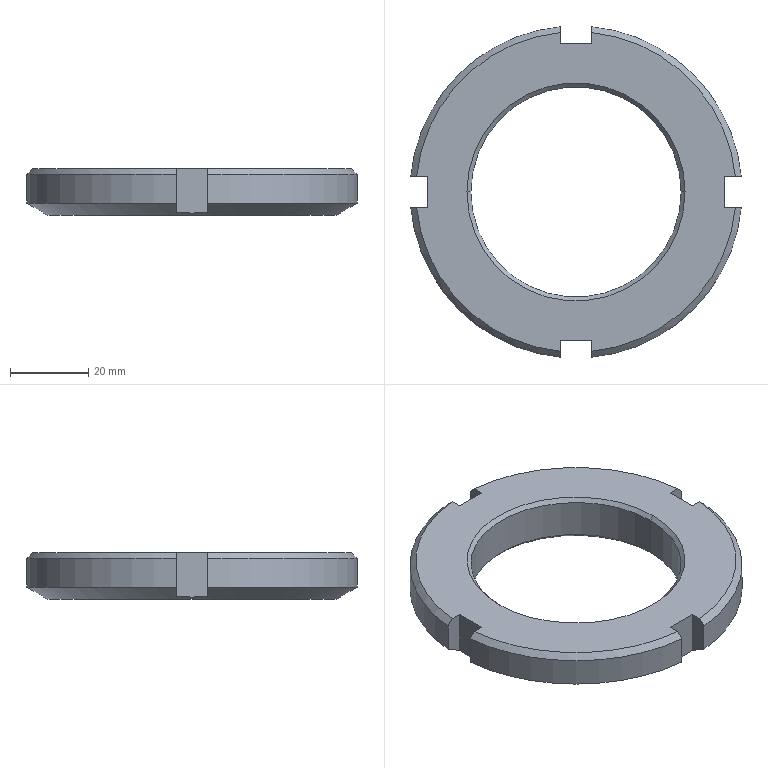Part | SolidWorks | features Chamfer 3, CirPattern 1, Cut 1, Extrusion 1 | 1 solid | 30 faces | box 84.623 x 84.623 x 12 mm | volume 36703 mm3 | plane 14 | cone 10 | cylinder 6 | commonest cylinder face diameters 85 x4 53.835 x2
STEP:
#1=CARTESIAN_POINT('',(-26.918,0.,11.));
#2=VERTEX_POINT('',#1);
#3=CARTESIAN_POINT('',(26.918,0.,11.));
#4=VERTEX_POINT('',#3);
#5=CARTESIAN_POINT('',(0.,0.,11.));
#6=DIRECTION('',(0.,0.,1.));
#7=DIRECTION('',(1.,0.,0.));
#8=AXIS2_PLACEMENT_3D('',#5,#6,#7);
#9=CIRCLE('',#8,26.918);
#10=EDGE_CURVE('',#2,#4,#9,.T.);
#11=ORIENTED_EDGE('',*,*,#10,.F.);
#12=CARTESIAN_POINT('',(-27.917,0.,12.));
#13=VERTEX_POINT('',#12);
#14=CARTESIAN_POINT('',(-26.918,0.,11.));
#15=DIRECTION('',(-0.7071,0.,0.7071));
#16=VECTOR('',#15,1000.);
#17=LINE('',#14,#16);
#18=EDGE_CURVE('',#2,#13,#17,.T.);
#19=ORIENTED_EDGE('',*,*,#18,.T.);
#20=CARTESIAN_POINT('',(27.917,0.,12.));
#21=VERTEX_POINT('',#20);
#22=CARTESIAN_POINT('',(0.,0.,12.));
#23=DIRECTION('',(0.,0.,-1.));
#24=DIRECTION('',(1.,0.,0.));
#25=AXIS2_PLACEMENT_3D('',#22,#23,#24);
#26=CIRCLE('',#25,27.917);
#27=EDGE_CURVE('',#21,#13,#26,.T.);
#28=ORIENTED_EDGE('',*,*,#27,.F.);
#29=CARTESIAN_POINT('',(26.918,0.,11.));
#30=DIRECTION('',(0.7071,0.,0.7071));
#31=VECTOR('',#30,1000.);
#32=LINE('',#29,#31);
#33=EDGE_CURVE('',#4,#21,#32,.T.);
#34=ORIENTED_EDGE('',*,*,#33,.F.);
#35=EDGE_LOOP('',(#11,#19,#28,#34));
#36=FACE_OUTER_BOUND('',#35,.T.);
#37=CARTESIAN_POINT('',(0.,0.,11.));
#38=DIRECTION('',(0.,0.,1.));
#39=DIRECTION('',(1.,0.,0.));
#40=AXIS2_PLACEMENT_3D('',#37,#38,#39);
#41=CONICAL_SURFACE('',#40,26.918,0.7854);
#42=ADVANCED_FACE('',(#36),#41,.F.);
#43=CARTESIAN_POINT('',(26.918,0.,1.));
#44=VERTEX_POINT('',#43);
#45=CARTESIAN_POINT('',(-26.918,0.,1.));
#46=VERTEX_POINT('',#45);
#47=CARTESIAN_POINT('',(0.,0.,1.));
#48=DIRECTION('',(0.,0.,-1.));
#49=DIRECTION('',(1.,0.,0.));
#50=AXIS2_PLACEMENT_3D('',#47,#48,#49);
#51=CIRCLE('',#50,26.918);
#52=EDGE_CURVE('',#44,#46,#51,.T.);
#53=ORIENTED_EDGE('',*,*,#52,.F.);
#54=CARTESIAN_POINT('',(27.917,0.,0.));
#55=VERTEX_POINT('',#54);
#56=CARTESIAN_POINT('',(27.917,0.,0.));
#57=DIRECTION('',(0.7071,0.,-0.7071));
#58=VECTOR('',#57,1000.);
#59=LINE('',#56,#58);
#60=EDGE_CURVE('',#44,#55,#59,.T.);
#61=ORIENTED_EDGE('',*,*,#60,.T.);
#62=CARTESIAN_POINT('',(-27.917,0.,0.));
#63=VERTEX_POINT('',#62);
#64=CARTESIAN_POINT('',(0.,0.,0.));
#65=DIRECTION('',(0.,0.,1.));
#66=DIRECTION('',(1.,0.,0.));
#67=AXIS2_PLACEMENT_3D('',#64,#65,#66);
#68=CIRCLE('',#67,27.917);
#69=EDGE_CURVE('',#63,#55,#68,.T.);
#70=ORIENTED_EDGE('',*,*,#69,.F.);
#71=CARTESIAN_POINT('',(-27.917,0.,0.));
#72=DIRECTION('',(-0.7071,0.,-0.7071));
#73=VECTOR('',#72,1000.);
#74=LINE('',#71,#73);
#75=EDGE_CURVE('',#46,#63,#74,.T.);
#76=ORIENTED_EDGE('',*,*,#75,.F.);
#77=EDGE_LOOP('',(#53,#61,#70,#76));
#78=FACE_OUTER_BOUND('',#77,.T.);
#79=CARTESIAN_POINT('',(0.,0.,0.));
#80=DIRECTION('',(0.,0.,-1.));
#81=DIRECTION('',(-1.,0.,0.));
#82=AXIS2_PLACEMENT_3D('',#79,#80,#81);
#83=CONICAL_SURFACE('',#82,27.917,0.7854);
#84=ADVANCED_FACE('',(#78),#83,.F.);
#85=CARTESIAN_POINT('',(-37.,0.,0.));
#86=VERTEX_POINT('',#85);
#87=CARTESIAN_POINT('',(37.,0.,0.));
#88=VERTEX_POINT('',#87);
#89=CARTESIAN_POINT('',(0.,0.,0.));
#90=DIRECTION('',(0.,0.,-1.));
#91=DIRECTION('',(1.,0.,0.));
#92=AXIS2_PLACEMENT_3D('',#89,#90,#91);
#93=CIRCLE('',#92,37.);
#94=EDGE_CURVE('',#86,#88,#93,.T.);
#95=ORIENTED_EDGE('',*,*,#94,.F.);
#96=CARTESIAN_POINT('',(-38.061,0.,0.6128));
#97=VERTEX_POINT('',#96);
#98=CARTESIAN_POINT('',(-42.5,0.,3.175));
#99=DIRECTION('',(-0.866,0.,0.5));
#100=VECTOR('',#99,1000.);
#101=LINE('',#98,#100);
#102=EDGE_CURVE('',#86,#97,#101,.T.);
#103=ORIENTED_EDGE('',*,*,#102,.T.);
#104=CARTESIAN_POINT('',(-38.061,4.,0.7338));
#105=VERTEX_POINT('',#104);
#106=CARTESIAN_POINT('',(-38.061,4.,0.7338));
#107=CARTESIAN_POINT('',(-38.061,2.67,0.6535));
#108=CARTESIAN_POINT('',(-38.061,1.337,0.6128));
#109=CARTESIAN_POINT('',(-38.061,0.,0.6128));
#110=B_SPLINE_CURVE_WITH_KNOTS('',3,(#106,#107,#108,#109),.UNSPECIFIED.,.F.,.F.,(4,4),(0.01039,0.01438),.UNSPECIFIED.);
#111=EDGE_CURVE('',#105,#97,#110,.T.);
#112=ORIENTED_EDGE('',*,*,#111,.F.);
#113=CARTESIAN_POINT('',(-42.311,4.,3.175));
#114=VERTEX_POINT('',#113);
#115=CARTESIAN_POINT('',(-42.311,4.,3.175));
#116=CARTESIAN_POINT('',(-42.064,4.,3.033));
#117=CARTESIAN_POINT('',(-41.816,4.,2.891));
#118=CARTESIAN_POINT('',(-41.569,4.,2.749));
#119=CARTESIAN_POINT('',(-40.4,4.,2.077));
#120=CARTESIAN_POINT('',(-39.231,4.,1.405));
#121=CARTESIAN_POINT('',(-38.061,4.,0.7338));
#122=B_SPLINE_CURVE_WITH_KNOTS('',3,(#115,#116,#117,#118,#119,#120,#121),.UNSPECIFIED.,.F.,.F.,(4,3,4),(0.009231,0.01009,0.01413),.UNSPECIFIED.);
#123=EDGE_CURVE('',#114,#105,#122,.T.);
#124=ORIENTED_EDGE('',*,*,#123,.F.);
#125=CARTESIAN_POINT('',(-4.,42.311,3.175));
#126=VERTEX_POINT('',#125);
#127=CARTESIAN_POINT('',(0.,0.,3.175));
#128=DIRECTION('',(0.,0.,1.));
#129=DIRECTION('',(1.,0.,0.));
#130=AXIS2_PLACEMENT_3D('',#127,#128,#129);
#131=CIRCLE('',#130,42.5);
#132=EDGE_CURVE('',#126,#114,#131,.T.);
#133=ORIENTED_EDGE('',*,*,#132,.F.);
#134=CARTESIAN_POINT('',(-4.,38.061,0.7338));
#135=VERTEX_POINT('',#134);
#136=CARTESIAN_POINT('',(-4.,38.061,0.7338));
#137=CARTESIAN_POINT('',(-4.,38.203,0.8152));
#138=CARTESIAN_POINT('',(-4.,38.345,0.8967));
#139=CARTESIAN_POINT('',(-4.,38.487,0.9781));
#140=CARTESIAN_POINT('',(-4.,39.762,1.71));
#141=CARTESIAN_POINT('',(-4.,41.037,2.443));
#142=CARTESIAN_POINT('',(-4.,42.311,3.175));
#143=B_SPLINE_CURVE_WITH_KNOTS('',3,(#136,#137,#138,#139,#140,#141,#142),.UNSPECIFIED.,.F.,.F.,(4,3,4),(0.009597,0.01009,0.0145),.UNSPECIFIED.);
#144=EDGE_CURVE('',#135,#126,#143,.T.);
#145=ORIENTED_EDGE('',*,*,#144,.F.);
#146=CARTESIAN_POINT('',(4.,38.061,0.7338));
#147=VERTEX_POINT('',#146);
#148=CARTESIAN_POINT('',(4.,38.061,0.7338));
#149=CARTESIAN_POINT('',(2.673,38.061,0.6537));
#150=CARTESIAN_POINT('',(1.343,38.061,0.613));
#151=CARTESIAN_POINT('',(-1.324,38.061,0.6126));
#152=CARTESIAN_POINT('',(-2.664,38.061,0.6532));
#153=CARTESIAN_POINT('',(-4.,38.061,0.7338));
#154=B_SPLINE_CURVE_WITH_KNOTS('',3,(#148,#149,#150,#151,#152,#153),.UNSPECIFIED.,.F.,.F.,(4,2,4),(0.01039,0.01437,0.01836),.UNSPECIFIED.);
#155=EDGE_CURVE('',#147,#135,#154,.T.);
#156=ORIENTED_EDGE('',*,*,#155,.F.);
#157=CARTESIAN_POINT('',(4.,42.311,3.175));
#158=VERTEX_POINT('',#157);
#159=CARTESIAN_POINT('',(4.,42.311,3.175));
#160=CARTESIAN_POINT('',(4.,41.037,2.443));
#161=CARTESIAN_POINT('',(4.,39.762,1.71));
#162=CARTESIAN_POINT('',(4.,38.487,0.9781));
#163=CARTESIAN_POINT('',(4.,38.345,0.8967));
#164=CARTESIAN_POINT('',(4.,38.203,0.8152));
#165=CARTESIAN_POINT('',(4.,38.061,0.7338));
#166=B_SPLINE_CURVE_WITH_KNOTS('',3,(#159,#160,#161,#162,#163,#164,#165),.UNSPECIFIED.,.F.,.F.,(4,3,4),(0.005677,0.01009,0.01058),.UNSPECIFIED.);
#167=EDGE_CURVE('',#158,#147,#166,.T.);
#168=ORIENTED_EDGE('',*,*,#167,.F.);
#169=CARTESIAN_POINT('',(42.311,4.,3.175));
#170=VERTEX_POINT('',#169);
#171=CARTESIAN_POINT('',(0.,0.,3.175));
#172=DIRECTION('',(0.,0.,1.));
#173=DIRECTION('',(1.,0.,0.));
#174=AXIS2_PLACEMENT_3D('',#171,#172,#173);
#175=CIRCLE('',#174,42.5);
#176=EDGE_CURVE('',#170,#158,#175,.T.);
#177=ORIENTED_EDGE('',*,*,#176,.F.);
#178=CARTESIAN_POINT('',(38.061,4.,0.7338));
#179=VERTEX_POINT('',#178);
#180=CARTESIAN_POINT('',(38.061,4.,0.7338));
#181=CARTESIAN_POINT('',(38.203,4.,0.8152));
#182=CARTESIAN_POINT('',(38.345,4.,0.8967));
#183=CARTESIAN_POINT('',(38.487,4.,0.9781));
#184=CARTESIAN_POINT('',(39.762,4.,1.71));
#185=CARTESIAN_POINT('',(41.037,4.,2.443));
#186=CARTESIAN_POINT('',(42.311,4.,3.175));
#187=B_SPLINE_CURVE_WITH_KNOTS('',3,(#180,#181,#182,#183,#184,#185,#186),.UNSPECIFIED.,.F.,.F.,(4,3,4),(0.009597,0.01009,0.0145),.UNSPECIFIED.);
#188=EDGE_CURVE('',#179,#170,#187,.T.);
#189=ORIENTED_EDGE('',*,*,#188,.F.);
#190=CARTESIAN_POINT('',(38.061,0.,0.6128));
#191=VERTEX_POINT('',#190);
#192=CARTESIAN_POINT('',(38.061,0.,0.6128));
#193=CARTESIAN_POINT('',(38.061,1.337,0.6128));
#194=CARTESIAN_POINT('',(38.061,2.67,0.6535));
#195=CARTESIAN_POINT('',(38.061,4.,0.7338));
#196=B_SPLINE_CURVE_WITH_KNOTS('',3,(#192,#193,#194,#195),.UNSPECIFIED.,.F.,.F.,(4,4),(0.02042,0.02442),.UNSPECIFIED.);
#197=EDGE_CURVE('',#191,#179,#196,.T.);
#198=ORIENTED_EDGE('',*,*,#197,.F.);
#199=CARTESIAN_POINT('',(42.5,0.,3.175));
#200=DIRECTION('',(0.866,0.,0.5));
#201=VECTOR('',#200,1000.);
#202=LINE('',#199,#201);
#203=EDGE_CURVE('',#88,#191,#202,.T.);
#204=ORIENTED_EDGE('',*,*,#203,.F.);
#205=EDGE_LOOP('',(#95,#103,#112,#124,#133,#145,#156,#168,#177,#189,#198,#204));
#206=FACE_OUTER_BOUND('',#205,.T.);
#207=CARTESIAN_POINT('',(0.,0.,3.175));
#208=DIRECTION('',(0.,0.,1.));
#209=DIRECTION('',(1.,0.,0.));
#210=AXIS2_PLACEMENT_3D('',#207,#208,#209);
#211=CONICAL_SURFACE('',#210,42.5,1.047);
#212=ADVANCED_FACE('',(#206),#211,.T.);
#213=ORIENTED_EDGE('',*,*,#10,.T.);
#214=CARTESIAN_POINT('',(26.918,0.,12.));
#215=DIRECTION('',(0.,0.,-1.));
#216=VECTOR('',#215,1000.);
#217=LINE('',#214,#216);
#218=EDGE_CURVE('',#4,#44,#217,.T.);
#219=ORIENTED_EDGE('',*,*,#218,.T.);
#220=ORIENTED_EDGE('',*,*,#52,.T.);
#221=CARTESIAN_POINT('',(-26.918,0.,12.));
#222=DIRECTION('',(0.,0.,-1.));
#223=VECTOR('',#222,1000.);
#224=LINE('',#221,#223);
#225=EDGE_CURVE('',#2,#46,#224,.T.);
#226=ORIENTED_EDGE('',*,*,#225,.F.);
#227=EDGE_LOOP('',(#213,#219,#220,#226));
#228=FACE_OUTER_BOUND('',#227,.T.);
#229=CARTESIAN_POINT('',(0.,0.,12.));
#230=DIRECTION('',(0.,0.,-1.));
#231=DIRECTION('',(-1.,0.,0.));
#232=AXIS2_PLACEMENT_3D('',#229,#230,#231);
#233=CYLINDRICAL_SURFACE('',#232,26.918);
#234=ADVANCED_FACE('',(#228),#233,.F.);
#235=CARTESIAN_POINT('',(4.,42.311,10.5));
#236=VERTEX_POINT('',#235);
#237=CARTESIAN_POINT('',(42.311,4.,10.5));
#238=VERTEX_POINT('',#237);
#239=CARTESIAN_POINT('',(0.,0.,10.5));
#240=DIRECTION('',(0.,0.,-1.));
#241=DIRECTION('',(1.,0.,0.));
#242=AXIS2_PLACEMENT_3D('',#239,#240,#241);
#243=CIRCLE('',#242,42.5);
#244=EDGE_CURVE('',#236,#238,#243,.T.);
#245=ORIENTED_EDGE('',*,*,#244,.T.);
#246=CARTESIAN_POINT('',(42.311,4.,0.));
#247=DIRECTION('',(0.,0.,1.));
#248=VECTOR('',#247,1000.);
#249=LINE('',#246,#248);
#250=EDGE_CURVE('',#170,#238,#249,.T.);
#251=ORIENTED_EDGE('',*,*,#250,.F.);
#252=ORIENTED_EDGE('',*,*,#176,.T.);
#253=CARTESIAN_POINT('',(4.,42.311,0.));
#254=DIRECTION('',(0.,0.,1.));
#255=VECTOR('',#254,1000.);
#256=LINE('',#253,#255);
#257=EDGE_CURVE('',#158,#236,#256,.T.);
#258=ORIENTED_EDGE('',*,*,#257,.T.);
#259=EDGE_LOOP('',(#245,#251,#252,#258));
#260=FACE_OUTER_BOUND('',#259,.T.);
#261=CARTESIAN_POINT('',(0.,0.,12.));
#262=DIRECTION('',(0.,0.,-1.));
#263=DIRECTION('',(-1.,0.,0.));
#264=AXIS2_PLACEMENT_3D('',#261,#262,#263);
#265=CYLINDRICAL_SURFACE('',#264,42.5);
#266=ADVANCED_FACE('',(#260),#265,.T.);
#267=CARTESIAN_POINT('',(40.804,4.,12.));
#268=VERTEX_POINT('',#267);
#269=CARTESIAN_POINT('',(42.311,4.,10.5));
#270=CARTESIAN_POINT('',(41.92,4.,10.89));
#271=CARTESIAN_POINT('',(41.528,4.,11.28));
#272=CARTESIAN_POINT('',(41.136,4.,11.67));
#273=CARTESIAN_POINT('',(41.025,4.,11.78));
#274=CARTESIAN_POINT('',(40.915,4.,11.89));
#275=CARTESIAN_POINT('',(40.804,4.,12.));
#276=B_SPLINE_CURVE_WITH_KNOTS('',3,(#269,#270,#271,#272,#273,#274,#275),.UNSPECIFIED.,.F.,.F.,(4,3,4),(0.007217,0.008875,0.009343),.UNSPECIFIED.);
#277=EDGE_CURVE('',#238,#268,#276,.T.);
#278=ORIENTED_EDGE('',*,*,#277,.F.);
#279=ORIENTED_EDGE('',*,*,#244,.F.);
#280=CARTESIAN_POINT('',(4.,40.804,12.));
#281=VERTEX_POINT('',#280);
#282=CARTESIAN_POINT('',(4.,40.804,12.));
#283=CARTESIAN_POINT('',(4.,40.915,11.89));
#284=CARTESIAN_POINT('',(4.,41.025,11.78));
#285=CARTESIAN_POINT('',(4.,41.136,11.67));
#286=CARTESIAN_POINT('',(4.,41.528,11.28));
#287=CARTESIAN_POINT('',(4.,41.92,10.89));
#288=CARTESIAN_POINT('',(4.,42.311,10.5));
#289=B_SPLINE_CURVE_WITH_KNOTS('',3,(#282,#283,#284,#285,#286,#287,#288),.UNSPECIFIED.,.F.,.F.,(4,3,4),(0.008408,0.008875,0.01053),.UNSPECIFIED.);
#290=EDGE_CURVE('',#281,#236,#289,.T.);
#291=ORIENTED_EDGE('',*,*,#290,.F.);
#292=CARTESIAN_POINT('',(0.,0.,12.));
#293=DIRECTION('',(0.,0.,1.));
#294=DIRECTION('',(1.,0.,0.));
#295=AXIS2_PLACEMENT_3D('',#292,#293,#294);
#296=CIRCLE('',#295,41.);
#297=EDGE_CURVE('',#268,#281,#296,.T.);
#298=ORIENTED_EDGE('',*,*,#297,.F.);
#299=EDGE_LOOP('',(#278,#279,#291,#298));
#300=FACE_OUTER_BOUND('',#299,.T.);
#301=CARTESIAN_POINT('',(0.,0.,12.));
#302=DIRECTION('',(0.,0.,-1.));
#303=DIRECTION('',(-1.,0.,0.));
#304=AXIS2_PLACEMENT_3D('',#301,#302,#303);
#305=CONICAL_SURFACE('',#304,41.,0.7854);
#306=ADVANCED_FACE('',(#300),#305,.T.);
#307=CARTESIAN_POINT('',(-42.311,4.,10.5));
#308=VERTEX_POINT('',#307);
#309=CARTESIAN_POINT('',(-4.,42.311,10.5));
#310=VERTEX_POINT('',#309);
#311=CARTESIAN_POINT('',(0.,0.,10.5));
#312=DIRECTION('',(0.,0.,-1.));
#313=DIRECTION('',(1.,0.,0.));
#314=AXIS2_PLACEMENT_3D('',#311,#312,#313);
#315=CIRCLE('',#314,42.5);
#316=EDGE_CURVE('',#308,#310,#315,.T.);
#317=ORIENTED_EDGE('',*,*,#316,.T.);
#318=CARTESIAN_POINT('',(-4.,42.311,0.));
#319=DIRECTION('',(0.,0.,1.));
#320=VECTOR('',#319,1000.);
#321=LINE('',#318,#320);
#322=EDGE_CURVE('',#126,#310,#321,.T.);
#323=ORIENTED_EDGE('',*,*,#322,.F.);
#324=ORIENTED_EDGE('',*,*,#132,.T.);
#325=CARTESIAN_POINT('',(-42.311,4.,0.));
#326=DIRECTION('',(0.,0.,1.));
#327=VECTOR('',#326,1000.);
#328=LINE('',#325,#327);
#329=EDGE_CURVE('',#114,#308,#328,.T.);
#330=ORIENTED_EDGE('',*,*,#329,.T.);
#331=EDGE_LOOP('',(#317,#323,#324,#330));
#332=FACE_OUTER_BOUND('',#331,.T.);
#333=CARTESIAN_POINT('',(0.,0.,12.));
#334=DIRECTION('',(0.,0.,-1.));
#335=DIRECTION('',(-1.,0.,0.));
#336=AXIS2_PLACEMENT_3D('',#333,#334,#335);
#337=CYLINDRICAL_SURFACE('',#336,42.5);
#338=ADVANCED_FACE('',(#332),#337,.T.);
#339=CARTESIAN_POINT('',(-4.,40.804,12.));
#340=VERTEX_POINT('',#339);
#341=CARTESIAN_POINT('',(-4.,42.311,10.5));
#342=CARTESIAN_POINT('',(-4.,41.92,10.89));
#343=CARTESIAN_POINT('',(-4.,41.528,11.28));
#344=CARTESIAN_POINT('',(-4.,41.136,11.67));
#345=CARTESIAN_POINT('',(-4.,41.025,11.78));
#346=CARTESIAN_POINT('',(-4.,40.915,11.89));
#347=CARTESIAN_POINT('',(-4.,40.804,12.));
#348=B_SPLINE_CURVE_WITH_KNOTS('',3,(#341,#342,#343,#344,#345,#346,#347),.UNSPECIFIED.,.F.,.F.,(4,3,4),(0.007217,0.008875,0.009343),.UNSPECIFIED.);
#349=EDGE_CURVE('',#310,#340,#348,.T.);
#350=ORIENTED_EDGE('',*,*,#349,.F.);
#351=ORIENTED_EDGE('',*,*,#316,.F.);
#352=CARTESIAN_POINT('',(-40.804,4.,12.));
#353=VERTEX_POINT('',#352);
#354=CARTESIAN_POINT('',(-40.804,4.,12.));
#355=CARTESIAN_POINT('',(-41.093,4.,11.713));
#356=CARTESIAN_POINT('',(-41.381,4.,11.426));
#357=CARTESIAN_POINT('',(-41.67,4.,11.139));
#358=CARTESIAN_POINT('',(-41.883,4.,10.926));
#359=CARTESIAN_POINT('',(-42.097,4.,10.713));
#360=CARTESIAN_POINT('',(-42.311,4.,10.5));
#361=B_SPLINE_CURVE_WITH_KNOTS('',3,(#354,#355,#356,#357,#358,#359,#360),.UNSPECIFIED.,.F.,.F.,(4,3,4),(0.007655,0.008875,0.009781),.UNSPECIFIED.);
#362=EDGE_CURVE('',#353,#308,#361,.T.);
#363=ORIENTED_EDGE('',*,*,#362,.F.);
#364=CARTESIAN_POINT('',(0.,0.,12.));
#365=DIRECTION('',(0.,0.,1.));
#366=DIRECTION('',(1.,0.,0.));
#367=AXIS2_PLACEMENT_3D('',#364,#365,#366);
#368=CIRCLE('',#367,41.);
#369=EDGE_CURVE('',#340,#353,#368,.T.);
#370=ORIENTED_EDGE('',*,*,#369,.F.);
#371=EDGE_LOOP('',(#350,#351,#363,#370));
#372=FACE_OUTER_BOUND('',#371,.T.);
#373=CARTESIAN_POINT('',(0.,0.,12.));
#374=DIRECTION('',(0.,0.,-1.));
#375=DIRECTION('',(-1.,0.,0.));
#376=AXIS2_PLACEMENT_3D('',#373,#374,#375);
#377=CONICAL_SURFACE('',#376,41.,0.7854);
#378=ADVANCED_FACE('',(#372),#377,.T.);
#379=CARTESIAN_POINT('',(-4.,-42.311,10.5));
#380=VERTEX_POINT('',#379);
#381=CARTESIAN_POINT('',(-42.311,-4.,10.5));
#382=VERTEX_POINT('',#381);
#383=CARTESIAN_POINT('',(0.,0.,10.5));
#384=DIRECTION('',(0.,0.,-1.));
#385=DIRECTION('',(1.,0.,0.));
#386=AXIS2_PLACEMENT_3D('',#383,#384,#385);
#387=CIRCLE('',#386,42.5);
#388=EDGE_CURVE('',#380,#382,#387,.T.);
#389=ORIENTED_EDGE('',*,*,#388,.T.);
#390=CARTESIAN_POINT('',(-42.311,-4.,3.175));
#391=VERTEX_POINT('',#390);
#392=CARTESIAN_POINT('',(-42.311,-4.,0.));
#393=DIRECTION('',(0.,0.,1.));
#394=VECTOR('',#393,1000.);
#395=LINE('',#392,#394);
#396=EDGE_CURVE('',#391,#382,#395,.T.);
#397=ORIENTED_EDGE('',*,*,#396,.F.);
#398=CARTESIAN_POINT('',(-4.,-42.311,3.175));
#399=VERTEX_POINT('',#398);
#400=CARTESIAN_POINT('',(0.,0.,3.175));
#401=DIRECTION('',(0.,0.,1.));
#402=DIRECTION('',(1.,0.,0.));
#403=AXIS2_PLACEMENT_3D('',#400,#401,#402);
#404=CIRCLE('',#403,42.5);
#405=EDGE_CURVE('',#391,#399,#404,.T.);
#406=ORIENTED_EDGE('',*,*,#405,.T.);
#407=CARTESIAN_POINT('',(-4.,-42.311,0.));
#408=DIRECTION('',(0.,0.,1.));
#409=VECTOR('',#408,1000.);
#410=LINE('',#407,#409);
#411=EDGE_CURVE('',#399,#380,#410,.T.);
#412=ORIENTED_EDGE('',*,*,#411,.T.);
#413=EDGE_LOOP('',(#389,#397,#406,#412));
#414=FACE_OUTER_BOUND('',#413,.T.);
#415=CARTESIAN_POINT('',(0.,0.,12.));
#416=DIRECTION('',(0.,0.,-1.));
#417=DIRECTION('',(-1.,0.,0.));
#418=AXIS2_PLACEMENT_3D('',#415,#416,#417);
#419=CYLINDRICAL_SURFACE('',#418,42.5);
#420=ADVANCED_FACE('',(#414),#419,.T.);
#421=CARTESIAN_POINT('',(-40.804,-4.,12.));
#422=VERTEX_POINT('',#421);
#423=CARTESIAN_POINT('',(-42.311,-4.,10.5));
#424=CARTESIAN_POINT('',(-42.097,-4.,10.713));
#425=CARTESIAN_POINT('',(-41.883,-4.,10.926));
#426=CARTESIAN_POINT('',(-41.67,-4.,11.139));
#427=CARTESIAN_POINT('',(-41.381,-4.,11.426));
#428=CARTESIAN_POINT('',(-41.093,-4.,11.713));
#429=CARTESIAN_POINT('',(-40.804,-4.,12.));
#430=B_SPLINE_CURVE_WITH_KNOTS('',3,(#423,#424,#425,#426,#427,#428,#429),.UNSPECIFIED.,.F.,.F.,(4,3,4),(0.00797,0.008875,0.0101),.UNSPECIFIED.);
#431=EDGE_CURVE('',#382,#422,#430,.T.);
#432=ORIENTED_EDGE('',*,*,#431,.F.);
#433=ORIENTED_EDGE('',*,*,#388,.F.);
#434=CARTESIAN_POINT('',(-4.,-40.804,12.));
#435=VERTEX_POINT('',#434);
#436=CARTESIAN_POINT('',(-4.,-40.804,12.));
#437=CARTESIAN_POINT('',(-4.,-41.093,11.713));
#438=CARTESIAN_POINT('',(-4.,-41.381,11.426));
#439=CARTESIAN_POINT('',(-4.,-41.67,11.139));
#440=CARTESIAN_POINT('',(-4.,-41.883,10.926));
#441=CARTESIAN_POINT('',(-4.,-42.097,10.713));
#442=CARTESIAN_POINT('',(-4.,-42.311,10.5));
#443=B_SPLINE_CURVE_WITH_KNOTS('',3,(#436,#437,#438,#439,#440,#441,#442),.UNSPECIFIED.,.F.,.F.,(4,3,4),(0.007655,0.008875,0.009781),.UNSPECIFIED.);
#444=EDGE_CURVE('',#435,#380,#443,.T.);
#445=ORIENTED_EDGE('',*,*,#444,.F.);
#446=CARTESIAN_POINT('',(0.,0.,12.));
#447=DIRECTION('',(0.,0.,1.));
#448=DIRECTION('',(1.,0.,0.));
#449=AXIS2_PLACEMENT_3D('',#446,#447,#448);
#450=CIRCLE('',#449,41.);
#451=EDGE_CURVE('',#422,#435,#450,.T.);
#452=ORIENTED_EDGE('',*,*,#451,.F.);
#453=EDGE_LOOP('',(#432,#433,#445,#452));
#454=FACE_OUTER_BOUND('',#453,.T.);
#455=CARTESIAN_POINT('',(0.,0.,12.));
#456=DIRECTION('',(0.,0.,-1.));
#457=DIRECTION('',(-1.,0.,0.));
#458=AXIS2_PLACEMENT_3D('',#455,#456,#457);
#459=CONICAL_SURFACE('',#458,41.,0.7854);
#460=ADVANCED_FACE('',(#454),#459,.T.);
#461=ORIENTED_EDGE('',*,*,#27,.T.);
#462=CARTESIAN_POINT('',(0.,0.,12.));
#463=DIRECTION('',(0.,0.,-1.));
#464=DIRECTION('',(1.,0.,0.));
#465=AXIS2_PLACEMENT_3D('',#462,#463,#464);
#466=CIRCLE('',#465,27.917);
#467=EDGE_CURVE('',#13,#21,#466,.T.);
#468=ORIENTED_EDGE('',*,*,#467,.T.);
#469=EDGE_LOOP('',(#461,#468));
#470=FACE_BOUND('',#469,.T.);
#471=CARTESIAN_POINT('',(38.061,4.,12.));
#472=VERTEX_POINT('',#471);
#473=CARTESIAN_POINT('',(38.061,4.,12.));
#474=DIRECTION('',(-1.,0.,0.));
#475=VECTOR('',#474,1000.);
#476=LINE('',#473,#475);
#477=EDGE_CURVE('',#268,#472,#476,.T.);
#478=ORIENTED_EDGE('',*,*,#477,.F.);
#479=ORIENTED_EDGE('',*,*,#297,.T.);
#480=CARTESIAN_POINT('',(4.,38.061,12.));
#481=VERTEX_POINT('',#480);
#482=CARTESIAN_POINT('',(4.,38.061,12.));
#483=DIRECTION('',(0.,1.,0.));
#484=VECTOR('',#483,1000.);
#485=LINE('',#482,#484);
#486=EDGE_CURVE('',#481,#281,#485,.T.);
#487=ORIENTED_EDGE('',*,*,#486,.F.);
#488=CARTESIAN_POINT('',(-4.,38.061,12.));
#489=VERTEX_POINT('',#488);
#490=CARTESIAN_POINT('',(4.,38.061,12.));
#491=DIRECTION('',(1.,0.,0.));
#492=VECTOR('',#491,1000.);
#493=LINE('',#490,#492);
#494=EDGE_CURVE('',#489,#481,#493,.T.);
#495=ORIENTED_EDGE('',*,*,#494,.F.);
#496=CARTESIAN_POINT('',(-4.,38.061,12.));
#497=DIRECTION('',(0.,-1.,0.));
#498=VECTOR('',#497,1000.);
#499=LINE('',#496,#498);
#500=EDGE_CURVE('',#340,#489,#499,.T.);
#501=ORIENTED_EDGE('',*,*,#500,.F.);
#502=ORIENTED_EDGE('',*,*,#369,.T.);
#503=CARTESIAN_POINT('',(-38.061,4.,12.));
#504=VERTEX_POINT('',#503);
#505=CARTESIAN_POINT('',(-38.061,4.,12.));
#506=DIRECTION('',(-1.,0.,0.));
#507=VECTOR('',#506,1000.);
#508=LINE('',#505,#507);
#509=EDGE_CURVE('',#504,#353,#508,.T.);
#510=ORIENTED_EDGE('',*,*,#509,.F.);
#511=CARTESIAN_POINT('',(-38.061,-4.,12.));
#512=VERTEX_POINT('',#511);
#513=CARTESIAN_POINT('',(-38.061,4.,12.));
#514=DIRECTION('',(0.,1.,0.));
#515=VECTOR('',#514,1000.);
#516=LINE('',#513,#515);
#517=EDGE_CURVE('',#512,#504,#516,.T.);
#518=ORIENTED_EDGE('',*,*,#517,.F.);
#519=CARTESIAN_POINT('',(-38.061,-4.,12.));
#520=DIRECTION('',(1.,0.,0.));
#521=VECTOR('',#520,1000.);
#522=LINE('',#519,#521);
#523=EDGE_CURVE('',#422,#512,#522,.T.);
#524=ORIENTED_EDGE('',*,*,#523,.F.);
#525=ORIENTED_EDGE('',*,*,#451,.T.);
#526=CARTESIAN_POINT('',(-4.,-38.061,12.));
#527=VERTEX_POINT('',#526);
#528=CARTESIAN_POINT('',(-4.,-38.061,12.));
#529=DIRECTION('',(0.,-1.,0.));
#530=VECTOR('',#529,1000.);
#531=LINE('',#528,#530);
#532=EDGE_CURVE('',#527,#435,#531,.T.);
#533=ORIENTED_EDGE('',*,*,#532,.F.);
#534=CARTESIAN_POINT('',(4.,-38.061,12.));
#535=VERTEX_POINT('',#534);
#536=CARTESIAN_POINT('',(-4.,-38.061,12.));
#537=DIRECTION('',(-1.,0.,0.));
#538=VECTOR('',#537,1000.);
#539=LINE('',#536,#538);
#540=EDGE_CURVE('',#535,#527,#539,.T.);
#541=ORIENTED_EDGE('',*,*,#540,.F.);
#542=CARTESIAN_POINT('',(4.,-40.804,12.));
#543=VERTEX_POINT('',#542);
#544=CARTESIAN_POINT('',(4.,-38.061,12.));
#545=DIRECTION('',(0.,1.,0.));
#546=VECTOR('',#545,1000.);
#547=LINE('',#544,#546);
#548=EDGE_CURVE('',#543,#535,#547,.T.);
#549=ORIENTED_EDGE('',*,*,#548,.F.);
#550=CARTESIAN_POINT('',(40.804,-4.,12.));
#551=VERTEX_POINT('',#550);
#552=CARTESIAN_POINT('',(0.,0.,12.));
#553=DIRECTION('',(0.,0.,1.));
#554=DIRECTION('',(1.,0.,0.));
#555=AXIS2_PLACEMENT_3D('',#552,#553,#554);
#556=CIRCLE('',#555,41.);
#557=EDGE_CURVE('',#543,#551,#556,.T.);
#558=ORIENTED_EDGE('',*,*,#557,.T.);
#559=CARTESIAN_POINT('',(38.061,-4.,12.));
#560=VERTEX_POINT('',#559);
#561=CARTESIAN_POINT('',(38.061,-4.,12.));
#562=DIRECTION('',(1.,0.,0.));
#563=VECTOR('',#562,1000.);
#564=LINE('',#561,#563);
#565=EDGE_CURVE('',#560,#551,#564,.T.);
#566=ORIENTED_EDGE('',*,*,#565,.F.);
#567=CARTESIAN_POINT('',(38.061,-4.,12.));
#568=DIRECTION('',(0.,-1.,0.));
#569=VECTOR('',#568,1000.);
#570=LINE('',#567,#569);
#571=EDGE_CURVE('',#472,#560,#570,.T.);
#572=ORIENTED_EDGE('',*,*,#571,.F.);
#573=EDGE_LOOP('',(#478,#479,#487,#495,#501,#502,#510,#518,#524,#525,#533,#541,#549,#558,#566,#572));
#574=FACE_OUTER_BOUND('',#573,.T.);
#575=CARTESIAN_POINT('',(0.,0.,12.));
#576=DIRECTION('',(0.,0.,1.));
#577=DIRECTION('',(1.,0.,0.));
#578=AXIS2_PLACEMENT_3D('',#575,#576,#577);
#579=PLANE('',#578);
#580=ADVANCED_FACE('',(#470,#574),#579,.T.);
#581=ORIENTED_EDGE('',*,*,#69,.T.);
#582=CARTESIAN_POINT('',(0.,0.,0.));
#583=DIRECTION('',(0.,0.,1.));
#584=DIRECTION('',(1.,0.,0.));
#585=AXIS2_PLACEMENT_3D('',#582,#583,#584);
#586=CIRCLE('',#585,27.917);
#587=EDGE_CURVE('',#55,#63,#586,.T.);
#588=ORIENTED_EDGE('',*,*,#587,.T.);
#589=EDGE_LOOP('',(#581,#588));
#590=FACE_BOUND('',#589,.T.);
#591=CARTESIAN_POINT('',(0.,0.,0.));
#592=DIRECTION('',(0.,0.,-1.));
#593=DIRECTION('',(1.,0.,0.));
#594=AXIS2_PLACEMENT_3D('',#591,#592,#593);
#595=CIRCLE('',#594,37.);
#596=EDGE_CURVE('',#88,#86,#595,.T.);
#597=ORIENTED_EDGE('',*,*,#596,.T.);
#598=ORIENTED_EDGE('',*,*,#94,.T.);
#599=EDGE_LOOP('',(#597,#598));
#600=FACE_OUTER_BOUND('',#599,.T.);
#601=CARTESIAN_POINT('',(0.,0.,0.));
#602=DIRECTION('',(0.,0.,1.));
#603=DIRECTION('',(1.,0.,0.));
#604=AXIS2_PLACEMENT_3D('',#601,#602,#603);
#605=PLANE('',#604);
#606=ADVANCED_FACE('',(#590,#600),#605,.F.);
#607=CARTESIAN_POINT('',(4.,-42.311,3.175));
#608=VERTEX_POINT('',#607);
#609=CARTESIAN_POINT('',(42.311,-4.,3.175));
#610=VERTEX_POINT('',#609);
#611=CARTESIAN_POINT('',(0.,0.,3.175));
#612=DIRECTION('',(0.,0.,1.));
#613=DIRECTION('',(1.,0.,0.));
#614=AXIS2_PLACEMENT_3D('',#611,#612,#613);
#615=CIRCLE('',#614,42.5);
#616=EDGE_CURVE('',#608,#610,#615,.T.);
#617=ORIENTED_EDGE('',*,*,#616,.T.);
#618=CARTESIAN_POINT('',(42.311,-4.,10.5));
#619=VERTEX_POINT('',#618);
#620=CARTESIAN_POINT('',(42.311,-4.,0.));
#621=DIRECTION('',(0.,0.,1.));
#622=VECTOR('',#621,1000.);
#623=LINE('',#620,#622);
#624=EDGE_CURVE('',#610,#619,#623,.T.);
#625=ORIENTED_EDGE('',*,*,#624,.T.);
#626=CARTESIAN_POINT('',(4.,-42.311,10.5));
#627=VERTEX_POINT('',#626);
#628=CARTESIAN_POINT('',(0.,0.,10.5));
#629=DIRECTION('',(0.,0.,-1.));
#630=DIRECTION('',(1.,0.,0.));
#631=AXIS2_PLACEMENT_3D('',#628,#629,#630);
#632=CIRCLE('',#631,42.5);
#633=EDGE_CURVE('',#619,#627,#632,.T.);
#634=ORIENTED_EDGE('',*,*,#633,.T.);
#635=CARTESIAN_POINT('',(4.,-42.311,0.));
#636=DIRECTION('',(0.,0.,1.));
#637=VECTOR('',#636,1000.);
#638=LINE('',#635,#637);
#639=EDGE_CURVE('',#608,#627,#638,.T.);
#640=ORIENTED_EDGE('',*,*,#639,.F.);
#641=EDGE_LOOP('',(#617,#625,#634,#640));
#642=FACE_OUTER_BOUND('',#641,.T.);
#643=CARTESIAN_POINT('',(0.,0.,12.));
#644=DIRECTION('',(0.,0.,-1.));
#645=DIRECTION('',(-1.,0.,0.));
#646=AXIS2_PLACEMENT_3D('',#643,#644,#645);
#647=CYLINDRICAL_SURFACE('',#646,42.5);
#648=ADVANCED_FACE('',(#642),#647,.T.);
#649=ORIENTED_EDGE('',*,*,#218,.F.);
#650=CARTESIAN_POINT('',(0.,0.,11.));
#651=DIRECTION('',(0.,0.,1.));
#652=DIRECTION('',(1.,0.,0.));
#653=AXIS2_PLACEMENT_3D('',#650,#651,#652);
#654=CIRCLE('',#653,26.918);
#655=EDGE_CURVE('',#4,#2,#654,.T.);
#656=ORIENTED_EDGE('',*,*,#655,.T.);
#657=ORIENTED_EDGE('',*,*,#225,.T.);
#658=CARTESIAN_POINT('',(0.,0.,1.));
#659=DIRECTION('',(0.,0.,-1.));
#660=DIRECTION('',(1.,0.,0.));
#661=AXIS2_PLACEMENT_3D('',#658,#659,#660);
#662=CIRCLE('',#661,26.918);
#663=EDGE_CURVE('',#46,#44,#662,.T.);
#664=ORIENTED_EDGE('',*,*,#663,.T.);
#665=EDGE_LOOP('',(#649,#656,#657,#664));
#666=FACE_OUTER_BOUND('',#665,.T.);
#667=CARTESIAN_POINT('',(0.,0.,12.));
#668=DIRECTION('',(0.,0.,-1.));
#669=DIRECTION('',(-1.,0.,0.));
#670=AXIS2_PLACEMENT_3D('',#667,#668,#669);
#671=CYLINDRICAL_SURFACE('',#670,26.918);
#672=ADVANCED_FACE('',(#666),#671,.F.);
#673=CARTESIAN_POINT('',(40.804,-4.,12.));
#674=CARTESIAN_POINT('',(40.915,-4.,11.89));
#675=CARTESIAN_POINT('',(41.025,-4.,11.78));
#676=CARTESIAN_POINT('',(41.136,-4.,11.67));
#677=CARTESIAN_POINT('',(41.528,-4.,11.28));
#678=CARTESIAN_POINT('',(41.92,-4.,10.89));
#679=CARTESIAN_POINT('',(42.311,-4.,10.5));
#680=B_SPLINE_CURVE_WITH_KNOTS('',3,(#673,#674,#675,#676,#677,#678,#679),.UNSPECIFIED.,.F.,.F.,(4,3,4),(0.008408,0.008875,0.01053),.UNSPECIFIED.);
#681=EDGE_CURVE('',#551,#619,#680,.T.);
#682=ORIENTED_EDGE('',*,*,#681,.F.);
#683=ORIENTED_EDGE('',*,*,#557,.F.);
#684=CARTESIAN_POINT('',(4.,-42.311,10.5));
#685=CARTESIAN_POINT('',(4.,-42.097,10.713));
#686=CARTESIAN_POINT('',(4.,-41.883,10.926));
#687=CARTESIAN_POINT('',(4.,-41.67,11.139));
#688=CARTESIAN_POINT('',(4.,-41.381,11.426));
#689=CARTESIAN_POINT('',(4.,-41.093,11.713));
#690=CARTESIAN_POINT('',(4.,-40.804,12.));
#691=B_SPLINE_CURVE_WITH_KNOTS('',3,(#684,#685,#686,#687,#688,#689,#690),.UNSPECIFIED.,.F.,.F.,(4,3,4),(0.00797,0.008875,0.0101),.UNSPECIFIED.);
#692=EDGE_CURVE('',#627,#543,#691,.T.);
#693=ORIENTED_EDGE('',*,*,#692,.F.);
#694=ORIENTED_EDGE('',*,*,#633,.F.);
#695=EDGE_LOOP('',(#682,#683,#693,#694));
#696=FACE_OUTER_BOUND('',#695,.T.);
#697=CARTESIAN_POINT('',(0.,0.,12.));
#698=DIRECTION('',(0.,0.,-1.));
#699=DIRECTION('',(-1.,0.,0.));
#700=AXIS2_PLACEMENT_3D('',#697,#698,#699);
#701=CONICAL_SURFACE('',#700,41.,0.7854);
#702=ADVANCED_FACE('',(#696),#701,.T.);
#703=ORIENTED_EDGE('',*,*,#102,.F.);
#704=ORIENTED_EDGE('',*,*,#596,.F.);
#705=ORIENTED_EDGE('',*,*,#203,.T.);
#706=CARTESIAN_POINT('',(38.061,-4.,0.7338));
#707=VERTEX_POINT('',#706);
#708=CARTESIAN_POINT('',(38.061,-4.,0.7338));
#709=CARTESIAN_POINT('',(38.061,-2.667,0.6534));
#710=CARTESIAN_POINT('',(38.061,-1.331,0.6128));
#711=CARTESIAN_POINT('',(38.061,0.,0.6128));
#712=B_SPLINE_CURVE_WITH_KNOTS('',3,(#708,#709,#710,#711),.UNSPECIFIED.,.F.,.F.,(4,4),(0.01643,0.02042),.UNSPECIFIED.);
#713=EDGE_CURVE('',#707,#191,#712,.T.);
#714=ORIENTED_EDGE('',*,*,#713,.F.);
#715=CARTESIAN_POINT('',(42.311,-4.,3.175));
#716=CARTESIAN_POINT('',(41.037,-4.,2.443));
#717=CARTESIAN_POINT('',(39.762,-4.,1.71));
#718=CARTESIAN_POINT('',(38.487,-4.,0.9781));
#719=CARTESIAN_POINT('',(38.345,-4.,0.8967));
#720=CARTESIAN_POINT('',(38.203,-4.,0.8152));
#721=CARTESIAN_POINT('',(38.061,-4.,0.7338));
#722=B_SPLINE_CURVE_WITH_KNOTS('',3,(#715,#716,#717,#718,#719,#720,#721),.UNSPECIFIED.,.F.,.F.,(4,3,4),(0.005677,0.01009,0.01058),.UNSPECIFIED.);
#723=EDGE_CURVE('',#610,#707,#722,.T.);
#724=ORIENTED_EDGE('',*,*,#723,.F.);
#725=ORIENTED_EDGE('',*,*,#616,.F.);
#726=CARTESIAN_POINT('',(4.,-38.061,0.7338));
#727=VERTEX_POINT('',#726);
#728=CARTESIAN_POINT('',(4.,-38.061,0.7338));
#729=CARTESIAN_POINT('',(4.,-39.231,1.405));
#730=CARTESIAN_POINT('',(4.,-40.4,2.077));
#731=CARTESIAN_POINT('',(4.,-41.569,2.749));
#732=CARTESIAN_POINT('',(4.,-41.816,2.891));
#733=CARTESIAN_POINT('',(4.,-42.064,3.033));
#734=CARTESIAN_POINT('',(4.,-42.311,3.175));
#735=B_SPLINE_CURVE_WITH_KNOTS('',3,(#728,#729,#730,#731,#732,#733,#734),.UNSPECIFIED.,.F.,.F.,(4,3,4),(0.006042,0.01009,0.01094),.UNSPECIFIED.);
#736=EDGE_CURVE('',#727,#608,#735,.T.);
#737=ORIENTED_EDGE('',*,*,#736,.F.);
#738=CARTESIAN_POINT('',(-4.,-38.061,0.7338));
#739=VERTEX_POINT('',#738);
#740=CARTESIAN_POINT('',(-4.,-38.061,0.7338));
#741=CARTESIAN_POINT('',(-2.664,-38.061,0.6532));
#742=CARTESIAN_POINT('',(-1.324,-38.061,0.6126));
#743=CARTESIAN_POINT('',(1.343,-38.061,0.613));
#744=CARTESIAN_POINT('',(2.673,-38.061,0.6537));
#745=CARTESIAN_POINT('',(4.,-38.061,0.7338));
#746=B_SPLINE_CURVE_WITH_KNOTS('',3,(#740,#741,#742,#743,#744,#745),.UNSPECIFIED.,.F.,.F.,(4,2,4),(0.01643,0.02042,0.02442),.UNSPECIFIED.);
#747=EDGE_CURVE('',#739,#727,#746,.T.);
#748=ORIENTED_EDGE('',*,*,#747,.F.);
#749=CARTESIAN_POINT('',(-4.,-42.311,3.175));
#750=CARTESIAN_POINT('',(-4.,-42.064,3.033));
#751=CARTESIAN_POINT('',(-4.,-41.816,2.891));
#752=CARTESIAN_POINT('',(-4.,-41.569,2.749));
#753=CARTESIAN_POINT('',(-4.,-40.4,2.077));
#754=CARTESIAN_POINT('',(-4.,-39.231,1.405));
#755=CARTESIAN_POINT('',(-4.,-38.061,0.7338));
#756=B_SPLINE_CURVE_WITH_KNOTS('',3,(#749,#750,#751,#752,#753,#754,#755),.UNSPECIFIED.,.F.,.F.,(4,3,4),(0.009231,0.01009,0.01413),.UNSPECIFIED.);
#757=EDGE_CURVE('',#399,#739,#756,.T.);
#758=ORIENTED_EDGE('',*,*,#757,.F.);
#759=ORIENTED_EDGE('',*,*,#405,.F.);
#760=CARTESIAN_POINT('',(-38.061,-4.,0.7338));
#761=VERTEX_POINT('',#760);
#762=CARTESIAN_POINT('',(-38.061,-4.,0.7338));
#763=CARTESIAN_POINT('',(-39.231,-4.,1.405));
#764=CARTESIAN_POINT('',(-40.4,-4.,2.077));
#765=CARTESIAN_POINT('',(-41.569,-4.,2.749));
#766=CARTESIAN_POINT('',(-41.816,-4.,2.891));
#767=CARTESIAN_POINT('',(-42.064,-4.,3.033));
#768=CARTESIAN_POINT('',(-42.311,-4.,3.175));
#769=B_SPLINE_CURVE_WITH_KNOTS('',3,(#762,#763,#764,#765,#766,#767,#768),.UNSPECIFIED.,.F.,.F.,(4,3,4),(0.006042,0.01009,0.01094),.UNSPECIFIED.);
#770=EDGE_CURVE('',#761,#391,#769,.T.);
#771=ORIENTED_EDGE('',*,*,#770,.F.);
#772=CARTESIAN_POINT('',(-38.061,0.,0.6128));
#773=CARTESIAN_POINT('',(-38.061,-1.331,0.6128));
#774=CARTESIAN_POINT('',(-38.061,-2.667,0.6534));
#775=CARTESIAN_POINT('',(-38.061,-4.,0.7338));
#776=B_SPLINE_CURVE_WITH_KNOTS('',3,(#772,#773,#774,#775),.UNSPECIFIED.,.F.,.F.,(4,4),(0.01438,0.01836),.UNSPECIFIED.);
#777=EDGE_CURVE('',#97,#761,#776,.T.);
#778=ORIENTED_EDGE('',*,*,#777,.F.);
#779=EDGE_LOOP('',(#703,#704,#705,#714,#724,#725,#737,#748,#758,#759,#771,#778));
#780=FACE_OUTER_BOUND('',#779,.T.);
#781=CARTESIAN_POINT('',(0.,0.,3.175));
#782=DIRECTION('',(0.,0.,1.));
#783=DIRECTION('',(1.,0.,0.));
#784=AXIS2_PLACEMENT_3D('',#781,#782,#783);
#785=CONICAL_SURFACE('',#784,42.5,1.047);
#786=ADVANCED_FACE('',(#780),#785,.T.);
#787=ORIENTED_EDGE('',*,*,#747,.T.);
#788=CARTESIAN_POINT('',(4.,-38.061,0.));
#789=DIRECTION('',(0.,0.,1.));
#790=VECTOR('',#789,1000.);
#791=LINE('',#788,#790);
#792=EDGE_CURVE('',#727,#535,#791,.T.);
#793=ORIENTED_EDGE('',*,*,#792,.T.);
#794=ORIENTED_EDGE('',*,*,#540,.T.);
#795=CARTESIAN_POINT('',(-4.,-38.061,0.));
#796=DIRECTION('',(0.,0.,1.));
#797=VECTOR('',#796,1000.);
#798=LINE('',#795,#797);
#799=EDGE_CURVE('',#739,#527,#798,.T.);
#800=ORIENTED_EDGE('',*,*,#799,.F.);
#801=EDGE_LOOP('',(#787,#793,#794,#800));
#802=FACE_OUTER_BOUND('',#801,.T.);
#803=CARTESIAN_POINT('',(-4.,-38.061,0.));
#804=DIRECTION('',(0.,1.,0.));
#805=DIRECTION('',(0.,0.,1.));
#806=AXIS2_PLACEMENT_3D('',#803,#804,#805);
#807=PLANE('',#806);
#808=ADVANCED_FACE('',(#802),#807,.F.);
#809=ORIENTED_EDGE('',*,*,#692,.T.);
#810=ORIENTED_EDGE('',*,*,#548,.T.);
#811=ORIENTED_EDGE('',*,*,#792,.F.);
#812=ORIENTED_EDGE('',*,*,#736,.T.);
#813=ORIENTED_EDGE('',*,*,#639,.T.);
#814=EDGE_LOOP('',(#809,#810,#811,#812,#813));
#815=FACE_OUTER_BOUND('',#814,.T.);
#816=CARTESIAN_POINT('',(4.,-38.061,0.));
#817=DIRECTION('',(1.,0.,0.));
#818=DIRECTION('',(0.,1.,0.));
#819=AXIS2_PLACEMENT_3D('',#816,#817,#818);
#820=PLANE('',#819);
#821=ADVANCED_FACE('',(#815),#820,.F.);
#822=ORIENTED_EDGE('',*,*,#444,.T.);
#823=ORIENTED_EDGE('',*,*,#411,.F.);
#824=ORIENTED_EDGE('',*,*,#757,.T.);
#825=ORIENTED_EDGE('',*,*,#799,.T.);
#826=ORIENTED_EDGE('',*,*,#532,.T.);
#827=EDGE_LOOP('',(#822,#823,#824,#825,#826));
#828=FACE_OUTER_BOUND('',#827,.T.);
#829=CARTESIAN_POINT('',(-4.,-38.061,0.));
#830=DIRECTION('',(-1.,0.,0.));
#831=DIRECTION('',(0.,0.,1.));
#832=AXIS2_PLACEMENT_3D('',#829,#830,#831);
#833=PLANE('',#832);
#834=ADVANCED_FACE('',(#828),#833,.F.);
#835=ORIENTED_EDGE('',*,*,#111,.T.);
#836=ORIENTED_EDGE('',*,*,#777,.T.);
#837=CARTESIAN_POINT('',(-38.061,-4.,0.));
#838=DIRECTION('',(0.,0.,1.));
#839=VECTOR('',#838,1000.);
#840=LINE('',#837,#839);
#841=EDGE_CURVE('',#761,#512,#840,.T.);
#842=ORIENTED_EDGE('',*,*,#841,.T.);
#843=ORIENTED_EDGE('',*,*,#517,.T.);
#844=CARTESIAN_POINT('',(-38.061,4.,0.));
#845=DIRECTION('',(0.,0.,1.));
#846=VECTOR('',#845,1000.);
#847=LINE('',#844,#846);
#848=EDGE_CURVE('',#105,#504,#847,.T.);
#849=ORIENTED_EDGE('',*,*,#848,.F.);
#850=EDGE_LOOP('',(#835,#836,#842,#843,#849));
#851=FACE_OUTER_BOUND('',#850,.T.);
#852=CARTESIAN_POINT('',(-38.061,4.,0.));
#853=DIRECTION('',(1.,0.,0.));
#854=DIRECTION('',(0.,1.,0.));
#855=AXIS2_PLACEMENT_3D('',#852,#853,#854);
#856=PLANE('',#855);
#857=ADVANCED_FACE('',(#851),#856,.F.);
#858=ORIENTED_EDGE('',*,*,#431,.T.);
#859=ORIENTED_EDGE('',*,*,#523,.T.);
#860=ORIENTED_EDGE('',*,*,#841,.F.);
#861=ORIENTED_EDGE('',*,*,#770,.T.);
#862=ORIENTED_EDGE('',*,*,#396,.T.);
#863=EDGE_LOOP('',(#858,#859,#860,#861,#862));
#864=FACE_OUTER_BOUND('',#863,.T.);
#865=CARTESIAN_POINT('',(-38.061,-4.,0.));
#866=DIRECTION('',(0.,-1.,0.));
#867=DIRECTION('',(1.,0.,0.));
#868=AXIS2_PLACEMENT_3D('',#865,#866,#867);
#869=PLANE('',#868);
#870=ADVANCED_FACE('',(#864),#869,.F.);
#871=ORIENTED_EDGE('',*,*,#362,.T.);
#872=ORIENTED_EDGE('',*,*,#329,.F.);
#873=ORIENTED_EDGE('',*,*,#123,.T.);
#874=ORIENTED_EDGE('',*,*,#848,.T.);
#875=ORIENTED_EDGE('',*,*,#509,.T.);
#876=EDGE_LOOP('',(#871,#872,#873,#874,#875));
#877=FACE_OUTER_BOUND('',#876,.T.);
#878=CARTESIAN_POINT('',(-38.061,4.,0.));
#879=DIRECTION('',(0.,1.,0.));
#880=DIRECTION('',(-1.,0.,0.));
#881=AXIS2_PLACEMENT_3D('',#878,#879,#880);
#882=PLANE('',#881);
#883=ADVANCED_FACE('',(#877),#882,.F.);
#884=ORIENTED_EDGE('',*,*,#155,.T.);
#885=CARTESIAN_POINT('',(-4.,38.061,0.));
#886=DIRECTION('',(0.,0.,1.));
#887=VECTOR('',#886,1000.);
#888=LINE('',#885,#887);
#889=EDGE_CURVE('',#135,#489,#888,.T.);
#890=ORIENTED_EDGE('',*,*,#889,.T.);
#891=ORIENTED_EDGE('',*,*,#494,.T.);
#892=CARTESIAN_POINT('',(4.,38.061,0.));
#893=DIRECTION('',(0.,0.,1.));
#894=VECTOR('',#893,1000.);
#895=LINE('',#892,#894);
#896=EDGE_CURVE('',#147,#481,#895,.T.);
#897=ORIENTED_EDGE('',*,*,#896,.F.);
#898=EDGE_LOOP('',(#884,#890,#891,#897));
#899=FACE_OUTER_BOUND('',#898,.T.);
#900=CARTESIAN_POINT('',(4.,38.061,0.));
#901=DIRECTION('',(0.,-1.,0.));
#902=DIRECTION('',(1.,0.,0.));
#903=AXIS2_PLACEMENT_3D('',#900,#901,#902);
#904=PLANE('',#903);
#905=ADVANCED_FACE('',(#899),#904,.F.);
#906=ORIENTED_EDGE('',*,*,#349,.T.);
#907=ORIENTED_EDGE('',*,*,#500,.T.);
#908=ORIENTED_EDGE('',*,*,#889,.F.);
#909=ORIENTED_EDGE('',*,*,#144,.T.);
#910=ORIENTED_EDGE('',*,*,#322,.T.);
#911=EDGE_LOOP('',(#906,#907,#908,#909,#910));
#912=FACE_OUTER_BOUND('',#911,.T.);
#913=CARTESIAN_POINT('',(-4.,38.061,0.));
#914=DIRECTION('',(-1.,0.,0.));
#915=DIRECTION('',(0.,-1.,0.));
#916=AXIS2_PLACEMENT_3D('',#913,#914,#915);
#917=PLANE('',#916);
#918=ADVANCED_FACE('',(#912),#917,.F.);
#919=ORIENTED_EDGE('',*,*,#290,.T.);
#920=ORIENTED_EDGE('',*,*,#257,.F.);
#921=ORIENTED_EDGE('',*,*,#167,.T.);
#922=ORIENTED_EDGE('',*,*,#896,.T.);
#923=ORIENTED_EDGE('',*,*,#486,.T.);
#924=EDGE_LOOP('',(#919,#920,#921,#922,#923));
#925=FACE_OUTER_BOUND('',#924,.T.);
#926=CARTESIAN_POINT('',(4.,38.061,0.));
#927=DIRECTION('',(1.,0.,0.));
#928=DIRECTION('',(0.,1.,0.));
#929=AXIS2_PLACEMENT_3D('',#926,#927,#928);
#930=PLANE('',#929);
#931=ADVANCED_FACE('',(#925),#930,.F.);
#932=ORIENTED_EDGE('',*,*,#713,.T.);
#933=ORIENTED_EDGE('',*,*,#197,.T.);
#934=CARTESIAN_POINT('',(38.061,4.,0.));
#935=DIRECTION('',(0.,0.,1.));
#936=VECTOR('',#935,1000.);
#937=LINE('',#934,#936);
#938=EDGE_CURVE('',#179,#472,#937,.T.);
#939=ORIENTED_EDGE('',*,*,#938,.T.);
#940=ORIENTED_EDGE('',*,*,#571,.T.);
#941=CARTESIAN_POINT('',(38.061,-4.,0.));
#942=DIRECTION('',(0.,0.,1.));
#943=VECTOR('',#942,1000.);
#944=LINE('',#941,#943);
#945=EDGE_CURVE('',#707,#560,#944,.T.);
#946=ORIENTED_EDGE('',*,*,#945,.F.);
#947=EDGE_LOOP('',(#932,#933,#939,#940,#946));
#948=FACE_OUTER_BOUND('',#947,.T.);
#949=CARTESIAN_POINT('',(38.061,-4.,0.));
#950=DIRECTION('',(-1.,0.,0.));
#951=DIRECTION('',(0.,-1.,0.));
#952=AXIS2_PLACEMENT_3D('',#949,#950,#951);
#953=PLANE('',#952);
#954=ADVANCED_FACE('',(#948),#953,.F.);
#955=ORIENTED_EDGE('',*,*,#277,.T.);
#956=ORIENTED_EDGE('',*,*,#477,.T.);
#957=ORIENTED_EDGE('',*,*,#938,.F.);
#958=ORIENTED_EDGE('',*,*,#188,.T.);
#959=ORIENTED_EDGE('',*,*,#250,.T.);
#960=EDGE_LOOP('',(#955,#956,#957,#958,#959));
#961=FACE_OUTER_BOUND('',#960,.T.);
#962=CARTESIAN_POINT('',(38.061,4.,0.));
#963=DIRECTION('',(0.,1.,0.));
#964=DIRECTION('',(-1.,0.,0.));
#965=AXIS2_PLACEMENT_3D('',#962,#963,#964);
#966=PLANE('',#965);
#967=ADVANCED_FACE('',(#961),#966,.F.);
#968=ORIENTED_EDGE('',*,*,#681,.T.);
#969=ORIENTED_EDGE('',*,*,#624,.F.);
#970=ORIENTED_EDGE('',*,*,#723,.T.);
#971=ORIENTED_EDGE('',*,*,#945,.T.);
#972=ORIENTED_EDGE('',*,*,#565,.T.);
#973=EDGE_LOOP('',(#968,#969,#970,#971,#972));
#974=FACE_OUTER_BOUND('',#973,.T.);
#975=CARTESIAN_POINT('',(38.061,-4.,0.));
#976=DIRECTION('',(0.,-1.,0.));
#977=DIRECTION('',(1.,0.,0.));
#978=AXIS2_PLACEMENT_3D('',#975,#976,#977);
#979=PLANE('',#978);
#980=ADVANCED_FACE('',(#974),#979,.F.);
#981=ORIENTED_EDGE('',*,*,#60,.F.);
#982=ORIENTED_EDGE('',*,*,#663,.F.);
#983=ORIENTED_EDGE('',*,*,#75,.T.);
#984=ORIENTED_EDGE('',*,*,#587,.F.);
#985=EDGE_LOOP('',(#981,#982,#983,#984));
#986=FACE_OUTER_BOUND('',#985,.T.);
#987=CARTESIAN_POINT('',(0.,0.,0.));
#988=DIRECTION('',(0.,0.,-1.));
#989=DIRECTION('',(-1.,0.,0.));
#990=AXIS2_PLACEMENT_3D('',#987,#988,#989);
#991=CONICAL_SURFACE('',#990,27.917,0.7854);
#992=ADVANCED_FACE('',(#986),#991,.F.);
#993=ORIENTED_EDGE('',*,*,#18,.F.);
#994=ORIENTED_EDGE('',*,*,#655,.F.);
#995=ORIENTED_EDGE('',*,*,#33,.T.);
#996=ORIENTED_EDGE('',*,*,#467,.F.);
#997=EDGE_LOOP('',(#993,#994,#995,#996));
#998=FACE_OUTER_BOUND('',#997,.T.);
#999=CARTESIAN_POINT('',(0.,0.,11.));
#1000=DIRECTION('',(0.,0.,1.));
#1001=DIRECTION('',(1.,0.,0.));
#1002=AXIS2_PLACEMENT_3D('',#999,#1000,#1001);
#1003=CONICAL_SURFACE('',#1002,26.918,0.7854);
#1004=ADVANCED_FACE('',(#998),#1003,.F.);
#1005=CLOSED_SHELL('',(#42,#84,#212,#234,#266,#306,#338,#378,#420,#460,#580,#606,#648,#672,#702,#786,#808,#821,#834,#857,#870,#883,#905,#918,#931,#954,#967,#980,#992,#1004));
#1006=MANIFOLD_SOLID_BREP('',#1005);
#1007=CARTESIAN_POINT('',(0.,0.,0.));
#1008=DIRECTION('',(0.,0.,1.));
#1009=DIRECTION('',(1.,0.,0.));
#1010=AXIS2_PLACEMENT_3D('',#1007,#1008,#1009);
#1011=(LENGTH_UNIT()NAMED_UNIT(*)SI_UNIT(.MILLI.,.METRE.));
#1012=UNCERTAINTY_MEASURE_WITH_UNIT(LENGTH_MEASURE(0.00001),#1011,'','');
#1013=(NAMED_UNIT(*)PLANE_ANGLE_UNIT()SI_UNIT($,.RADIAN.));
#1014=(NAMED_UNIT(*)SI_UNIT($,.STERADIAN.)SOLID_ANGLE_UNIT());
#1015=(GEOMETRIC_REPRESENTATION_CONTEXT(3)GLOBAL_UNCERTAINTY_ASSIGNED_CONTEXT((#1012))GLOBAL_UNIT_ASSIGNED_CONTEXT((#1011,#1013,#1014))REPRESENTATION_CONTEXT('',''));
#1016=ADVANCED_BREP_SHAPE_REPRESENTATION('',(#1006,#1010),#1015);